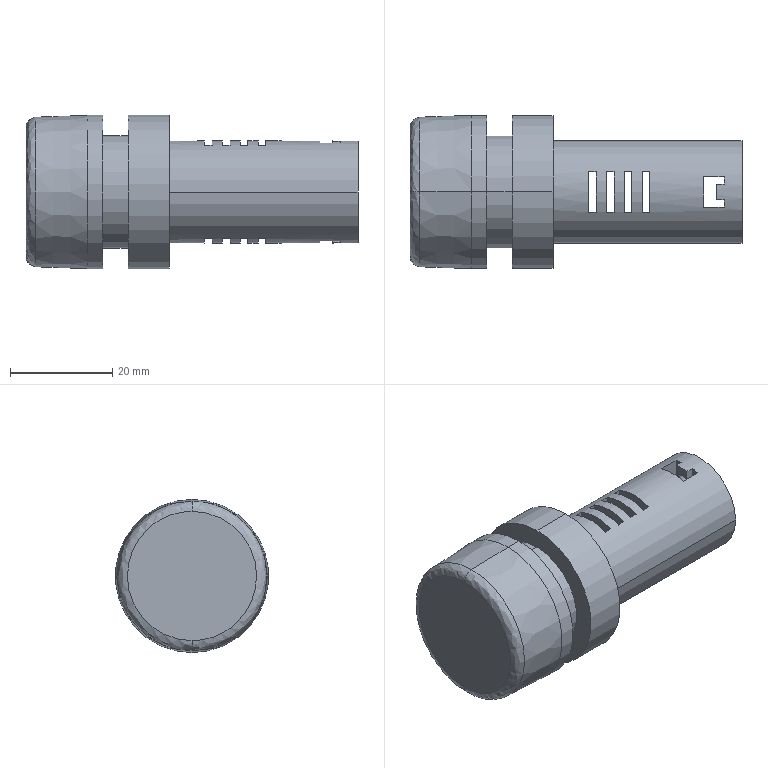Part | SolidWorks | features BaseBody 2 | 2 solids | 61 faces | box 65 x 30 x 30 mm | volume 34522 mm3 | plane 39 | cylinder 16 | cone 4 | spline 2 | commonest cylinder face diameters 4.5 x8 30 x4 20 x2 22 x2